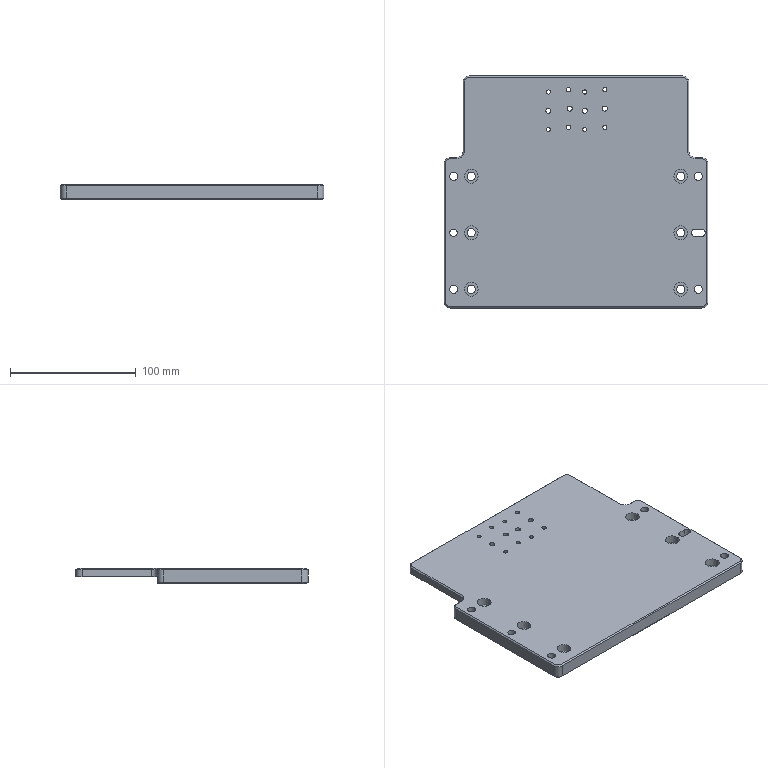Part | STEP file | 04-16 support bracket | 1 solid | 114 faces | box 210 x 185 x 12 mm | volume 371690 mm3 | cylinder 69 | plane 31 | cone 14 | commonest cylinder face diameters 3.3 x16 6.6 x12 11 x12 4 x8 6.5 x8 10 x8